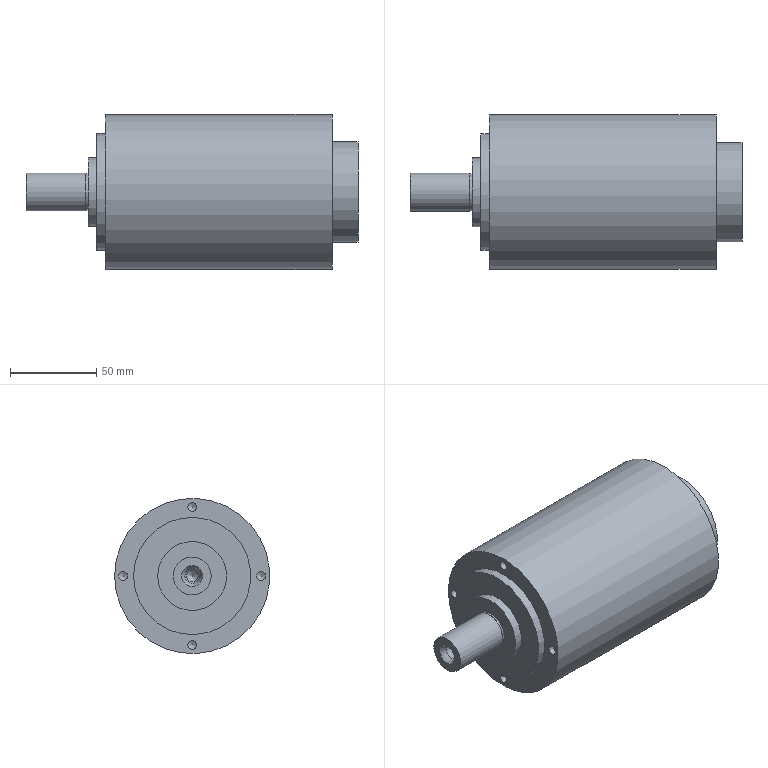Part | STEP file | SOLID | 1 solid | 37 faces | box 192.5 x 90 x 90 mm | volume 903685 mm3 | cylinder 16 | plane 13 | cone 7 | torus 1 | commonest cylinder face diameters 5.1 x4 24 x2 6.8 x1 8.4 x1 21.6 x1 22 x1